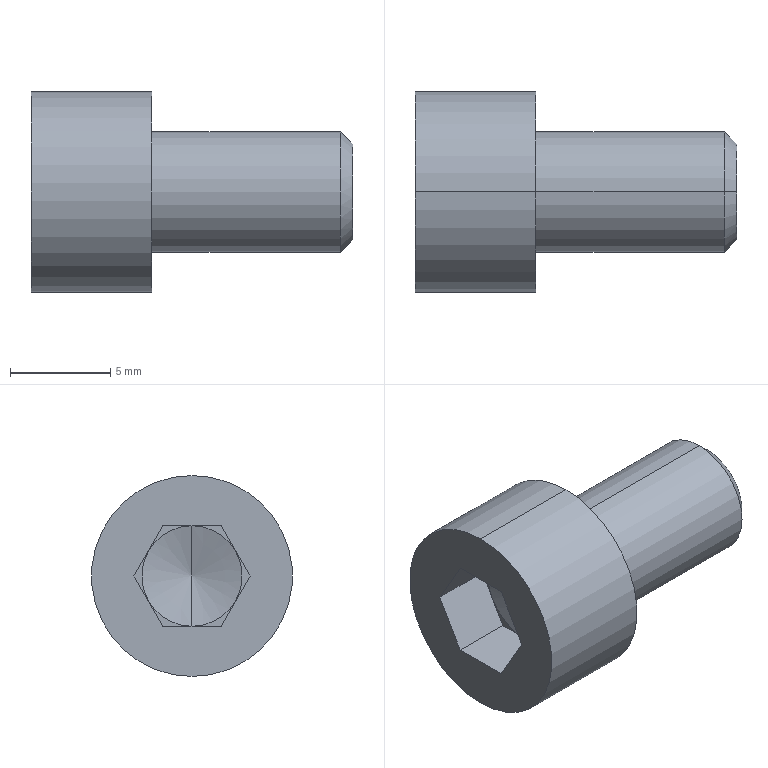Part | STEP file | CB6X1-10-A10-E6-B5 | 1 solid | 23 faces | box 16 x 10 x 10 mm | volume 681.341 mm3 | plane 15 | cylinder 4 | cone 4 | commonest cylinder face diameters 6 x2 10 x2